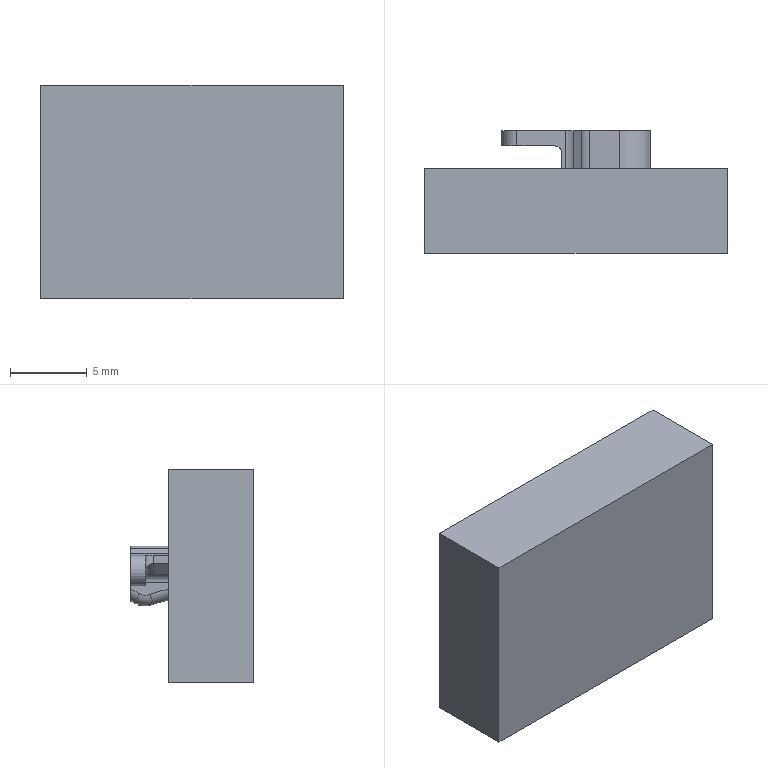NC program | NX | posted with a generic post | part box 19.7 x 8 x 13.91 mm
Lines 9382 to 10432 of 12778:
(ZLEVEL_PROFILE_COPY_1_COPY , TOOL : D1)
N18726 T05 M6
N18728 G54
N18730 G17 G0 G90 X-2.867 Y1.455 B0. C0. S7000 M3
N18732 G43 Z30. H5
N18734 Z-0.02
N18736 G94 G1 X-2.98 Y1.337 F1000.
N18738 X-3.008 Y1.313
N18740 X-3.017 Y1.276
N18742 X-3.004 Y1.24
N18744 G2 X-2.95 Y0.861 R1.381 F850.
N18746 G1 Y0.395
N18748 X-2.095
N18750 X-2.058 Y0.392
N18752 X-2.025 Y0.411
N18754 X-2.009 Y0.445
N18756 X-1.922 Y0.595
N18758 G0 X-2.862 Y1.454 Z-0.04
N18760 G1 X-2.976 Y1.338 F1000.
N18762 X-3.005 Y1.313
N18764 X-3.015 Y1.276
N18766 X-3.001 Y1.241
N18768 G2 X-2.95 Y0.872 R1.386 F850.
N18770 G1 Y0.395
N18772 X-2.095
N18774 X-2.058 Y0.392
N18776 X-2.025 Y0.411
N18778 X-2.009 Y0.445
N18780 X-1.922 Y0.595
N18782 G0 X-2.858 Y1.453 Z-0.06
N18784 G1 X-2.973 Y1.338 F1000.
N18786 X-3.002 Y1.313
N18788 X-3.012 Y1.276
N18790 X-2.999 Y1.241
N18792 G2 X-2.95 Y0.883 R1.392 F850.
N18794 G1 Y0.395
N18796 X-2.095
N18798 X-2.058 Y0.392
N18800 X-2.025 Y0.411
N18802 X-2.009 Y0.445
N18804 X-1.922 Y0.595
N18806 G0 X-2.853 Y1.452 Z-0.08
N18808 G1 X-2.969 Y1.338 F1000.
N18810 X-2.998 Y1.314
N18812 X-3.008 Y1.277
N18814 X-2.995 Y1.241
N18816 G2 X-2.95 Y0.893 R1.365 F850.
N18818 G1 Y0.395
N18820 X-2.095
N18822 X-2.058 Y0.392
N18824 X-2.025 Y0.411
N18826 X-2.009 Y0.445
N18828 X-1.922 Y0.595
N18830 G0 X-2.85 Y1.452 Z-0.1
N18832 G1 X-2.966 Y1.338 F1000.
N18834 X-2.996 Y1.314
N18836 X-3.006 Y1.277
N18838 X-2.993 Y1.241
N18840 G2 X-2.95 Y0.904 R1.396 F850.
N18842 G1 Y0.395
N18844 X-2.095
N18846 X-2.058 Y0.392
N18848 X-2.025 Y0.411
N18850 X-2.009 Y0.445
N18852 X-1.922 Y0.595
N18854 G0 X-2.845 Y1.451 Z-0.12
N18856 G1 X-2.963 Y1.338 F1000.
N18858 X-2.992 Y1.314
N18860 X-3.003 Y1.277
N18862 X-2.991 Y1.242
N18864 G2 X-2.95 Y0.915 R1.401 F850.
N18866 G1 Y0.395
N18868 X-2.095
N18870 X-2.058 Y0.392
N18872 X-2.025 Y0.411
N18874 X-2.009 Y0.445
N18876 X-1.922 Y0.595
N18878 G0 X-2.841 Y1.45 Z-0.14
N18880 G1 X-2.96 Y1.338 F1000.
N18882 X-2.989 Y1.314
N18884 X-3. Y1.278
N18886 X-2.988 Y1.242
N18888 G2 X-2.95 Y0.926 R1.398 F850.
N18890 G1 Y0.395
N18892 X-2.095
N18894 X-2.058 Y0.392
N18896 X-2.025 Y0.411
N18898 X-2.009 Y0.445
N18900 X-1.922 Y0.595
N18902 G0 X-2.837 Y1.449 Z-0.16
N18904 G1 X-2.956 Y1.338 F1000.
N18906 X-2.986 Y1.315
N18908 X-2.997 Y1.278
N18910 X-2.985 Y1.242
N18912 G2 X-2.95 Y0.937 R1.395 F850.
N18914 G1 Y0.395
N18916 X-2.095
N18918 X-2.058 Y0.392
N18920 X-2.025 Y0.411
N18922 X-2.009 Y0.445
N18924 X-1.922 Y0.595
N18926 G0 X-2.833 Y1.448 Z-0.18
N18928 G1 X-2.953 Y1.338 F1000.
N18930 X-2.983 Y1.315
N18932 X-2.994 Y1.278
N18934 X-2.983 Y1.242
N18936 G2 X-2.95 Y0.948 R1.391 F850.
N18938 G1 Y0.395
N18940 X-2.095
N18942 X-2.058 Y0.392
N18944 X-2.025 Y0.411
N18946 X-2.009 Y0.445
N18948 X-1.922 Y0.595
N18950 G0 X-2.828 Y1.447 Z-0.2
N18952 G1 X-2.949 Y1.338 F1000.
N18954 X-2.979 Y1.315
N18956 X-2.991 Y1.279
N18958 X-2.98 Y1.243
N18960 G2 X-2.95 Y0.959 R1.369 F850.
N18962 G1 Y0.395
N18964 X-2.095
N18966 X-2.058 Y0.392
N18968 X-2.025 Y0.411
N18970 X-2.009 Y0.445
N18972 X-1.922 Y0.595
N18974 G0 X-2.824 Y1.445 Z-0.22
N18976 G1 X-2.946 Y1.338 F1000.
N18978 X-2.977 Y1.315
N18980 X-2.989 Y1.279
N18982 X-2.978 Y1.243
N18984 G2 X-2.95 Y0.97 R1.379 F850.
N18986 G1 Y0.395
N18988 X-2.095
N18990 X-2.058 Y0.392
N18992 X-2.025 Y0.411
N18994 X-2.009 Y0.445
N18996 X-1.922 Y0.595
N18998 G0 X-2.82 Y1.444 Z-0.24
N19000 G1 X-2.943 Y1.337 F1000.
N19002 X-2.974 Y1.315
N19004 X-2.986 Y1.279
N19006 X-2.976 Y1.243
N19008 G2 X-2.95 Y0.981 R1.376 F850.
N19010 G1 Y0.395
N19012 X-2.095
N19014 X-2.058 Y0.392
N19016 X-2.025 Y0.411
N19018 X-2.009 Y0.445
N19020 X-1.922 Y0.595
N19022 G0 X-2.817 Y1.443 Z-0.26
N19024 G1 X-2.94 Y1.337 F1000.
N19026 X-2.971 Y1.315
N19028 X-2.984 Y1.279
N19030 X-2.973 Y1.243
N19032 G2 X-2.95 Y0.992 R1.374 F850.
N19034 G1 Y0.395
N19036 X-2.095
N19038 X-2.058 Y0.392
N19040 X-2.025 Y0.411
N19042 X-2.009 Y0.445
N19044 X-1.922 Y0.595
N19046 G0 X-2.813 Y1.442 Z-0.28
N19048 G1 X-2.938 Y1.337 F1000.
N19050 X-2.969 Y1.315
N19052 X-2.981 Y1.279
N19054 X-2.972 Y1.243
N19056 G2 X-2.95 Y1.003 R1.375 F850.
N19058 G1 Y0.395
N19060 X-2.095
N19062 X-2.058 Y0.392
N19064 X-2.025 Y0.411
N19066 X-2.009 Y0.445
N19068 X-1.922 Y0.595
N19070 G0 X-2.808 Y1.44 Z-0.3
N19072 G1 X-2.933 Y1.337 F1000.
N19074 X-2.965 Y1.315
N19076 X-2.978 Y1.28
N19078 X-2.968 Y1.243
N19080 G2 X-2.95 Y1.014 R1.335 F850.
N19082 G1 Y0.395
N19084 X-2.095
N19086 X-2.058 Y0.392
N19088 X-2.025 Y0.411
N19090 X-2.009 Y0.445
N19092 X-1.922 Y0.595
N19094 G0 X-2.805 Y1.439 Z-0.32
N19096 G1 X-2.931 Y1.337 F1000.
N19098 X-2.962 Y1.316
N19100 X-2.976 Y1.28
N19102 X-2.967 Y1.243
N19104 G2 X-2.95 Y1.025 R1.337 F850.
N19106 G1 Y0.395
N19108 X-2.095
N19110 X-2.058 Y0.392
N19112 X-2.025 Y0.411
N19114 X-2.009 Y0.445
N19116 X-1.922 Y0.595
N19118 G0 X-2.804 Y1.439 Z-0.34
N19120 G1 X-2.93 Y1.337 F1000.
N19122 X-2.962 Y1.316
N19124 X-2.976 Y1.28
N19126 X-2.967 Y1.243
N19128 G2 X-2.95 Y1.036 R1.382 F850.
N19130 G1 Y0.395
N19132 X-2.095
N19134 X-2.058 Y0.392
N19136 X-2.025 Y0.411
N19138 X-2.009 Y0.445
N19140 X-1.922 Y0.595
N19142 G0 X-2.801 Y1.438 Z-0.36
N19144 G1 X-2.928 Y1.336 F1000.
N19146 X-2.96 Y1.316
N19148 X-2.974 Y1.28
N19150 X-2.965 Y1.243
N19152 X-2.944 Y1.146 F850.
N19154 X-2.95 Y1.047
N19156 Y0.395
N19158 X-2.095
N19160 X-2.058 Y0.392
N19162 X-2.025 Y0.411
N19164 X-2.009 Y0.445
N19166 X-1.922 Y0.595
N19168 G0 X-2.797 Y1.436 Z-0.38
N19170 G1 X-2.926 Y1.336 F1000.
N19172 X-2.957 Y1.316
N19174 X-2.972 Y1.28
N19176 X-2.963 Y1.243
N19178 X-2.944 Y1.151 F850.
N19180 X-2.95 Y1.058
N19182 Y0.395
N19184 X-2.095
N19186 X-2.058 Y0.392
N19188 X-2.025 Y0.411
N19190 X-2.009 Y0.445
N19192 X-1.922 Y0.595
N19194 G0 X-2.794 Y1.435 Z-0.4
N19196 G1 X-2.923 Y1.336 F1000.
N19198 X-2.955 Y1.316
N19200 X-2.97 Y1.28
N19202 X-2.961 Y1.243
N19204 X-2.943 Y1.157 F850.
N19206 X-2.95 Y1.069
N19208 Y0.395
N19210 X-2.095
N19212 X-2.058 Y0.392
N19214 X-2.025 Y0.411
N19216 X-2.009 Y0.445
N19218 X-1.922 Y0.595
N19220 G0 X-2.79 Y1.433 Z-0.42
N19222 G1 X-2.92 Y1.335 F1000.
N19224 X-2.952 Y1.316
N19226 X-2.967 Y1.28
N19228 X-2.959 Y1.244
N19230 X-2.942 Y1.162 F850.
N19232 X-2.95 Y1.079
N19234 Y0.395
N19236 X-2.095
N19238 X-2.058 Y0.392
N19240 X-2.025 Y0.411
N19242 X-2.009 Y0.445
N19244 X-1.922 Y0.595
N19246 G0 X-2.788 Y1.432 Z-0.44
N19248 G1 X-2.919 Y1.335 F1000.
N19250 X-2.951 Y1.316
N19252 X-2.966 Y1.281
N19254 X-2.958 Y1.244
N19256 X-2.95 Y1.09 F850.
N19258 Y0.395
N19260 X-2.095
N19262 X-2.058 Y0.392
N19264 X-2.025 Y0.411
N19266 X-2.009 Y0.445
N19268 X-1.922 Y0.595
N19270 G0 X-2.785 Y1.431 Z-0.46
N19272 G1 X-2.917 Y1.335 F1000.
N19274 X-2.949 Y1.316
N19276 X-2.965 Y1.281
N19278 X-2.957 Y1.244
N19280 X-2.95 Y1.101 F850.
N19282 Y0.395
N19284 X-2.095
N19286 X-2.058 Y0.392
N19288 X-2.025 Y0.411
N19290 X-2.009 Y0.445
N19292 X-1.922 Y0.595
N19294 G0 X-2.783 Y1.429 Z-0.48
N19296 G1 X-2.915 Y1.335 F1000.
N19298 X-2.948 Y1.316
N19300 X-2.963 Y1.281
N19302 X-2.956 Y1.244
N19304 X-2.95 Y1.112 F850.
N19306 Y0.395
N19308 X-2.095
N19310 X-2.058 Y0.392
N19312 X-2.025 Y0.411
N19314 X-2.009 Y0.445
N19316 X-1.922 Y0.595
N19318 G0 X-2.781 Y1.428 Z-0.5
N19320 G1 X-2.914 Y1.334 F1000.
N19322 X-2.946 Y1.315
N19324 X-2.962 Y1.281
N19326 X-2.956 Y1.244
N19328 X-2.95 Y1.123 F850.
N19330 Y0.395
N19332 X-2.095
N19334 X-2.058 Y0.392
N19336 X-2.025 Y0.411
N19338 X-2.009 Y0.445
N19340 X-1.922 Y0.595
N19342 G0 X-2.778 Y1.426 Z-0.52
N19344 G1 X-2.912 Y1.334 F1000.
N19346 X-2.944 Y1.315
N19348 X-2.961 Y1.281
N19350 X-2.954 Y1.244
N19352 X-2.95 Y1.134 F850.
N19354 Y0.395
N19356 X-2.095
N19358 X-2.058 Y0.392
N19360 X-2.025 Y0.411
N19362 X-2.009 Y0.445
N19364 X-1.922 Y0.595
N19366 G0 X-2.776 Y1.425 Z-0.54
N19368 G1 X-2.91 Y1.334 F1000.
N19370 X-2.943 Y1.315
N19372 X-2.96 Y1.281
N19374 X-2.954 Y1.244
N19376 X-2.95 Y1.145 F850.
N19378 Y0.395
N19380 X-2.095
N19382 X-2.058 Y0.392
N19384 X-2.025 Y0.411
N19386 X-2.009 Y0.445
N19388 X-1.922 Y0.595
N19390 G0 X-2.775 Y1.425 Z-0.56
N19392 G1 X-2.91 Y1.334 F1000.
N19394 X-2.943 Y1.315
N19396 X-2.959 Y1.281
N19398 X-2.953 Y1.244
N19400 X-2.95 Y1.156 F850.
N19402 Y0.395
N19404 X-2.095
N19406 X-2.058 Y0.392
N19408 X-2.025 Y0.411
N19410 X-2.009 Y0.445
N19412 X-1.922 Y0.595
N19414 G0 X-2.774 Y1.424 Z-0.58
N19416 G1 X-2.909 Y1.334 F1000.
N19418 X-2.942 Y1.315
N19420 X-2.959 Y1.281
N19422 X-2.953 Y1.244
N19424 X-2.95 Y1.166 F850.
N19426 Y0.395
N19428 X-2.095
N19430 X-2.058 Y0.392
N19432 X-2.025 Y0.411
N19434 X-2.009 Y0.445
N19436 X-1.922 Y0.595
N19438 G0 X-2.772 Y1.429 Z-0.6
N19440 G1 X-2.912 Y1.334 F1000.
N19442 X-2.945 Y1.315
N19444 X-2.961 Y1.281
N19446 X-2.955 Y1.244
N19448 X-2.95 Y1.176 F850.
N19450 Y0.395
N19452 X-2.095
N19454 X-2.058 Y0.392
N19456 X-2.025 Y0.411
N19458 X-2.009 Y0.445
N19460 X-1.922 Y0.595
N19462 G0 X-2.774 Y1.432 Z-0.62
N19464 G1 X-2.913 Y1.334 F1000.
N19466 X-2.946 Y1.316
N19468 X-2.962 Y1.281
N19470 X-2.955 Y1.244
N19472 X-2.95 Y1.186 F850.
N19474 Y0.395
N19476 X-2.095
N19478 X-2.058 Y0.392
N19480 X-2.025 Y0.411
N19482 X-2.009 Y0.445
N19484 X-1.922 Y0.595
N19486 G0 X-2.767 Y1.409 Z-0.64
N19488 G1 X-2.903 Y1.33 F1000.
N19490 X-2.938 Y1.315
N19492 X-2.957 Y1.281
N19494 X-2.953 Y1.244
N19496 Y1.222 F850.
N19498 X-2.95 Y1.195
N19500 Y0.395
N19502 X-2.095
N19504 X-2.058 Y0.392
N19506 X-2.025 Y0.411
N19508 X-2.009 Y0.445
N19510 X-1.922 Y0.595
N19512 G0 X-2.766 Y1.41 Z-0.66
N19514 G1 X-2.903 Y1.33 F1000.
N19516 X-2.938 Y1.315
N19518 X-2.957 Y1.281
N19520 X-2.953 Y1.244
N19522 Y1.222 F850.
N19524 X-2.95 Y1.203
N19526 Y0.395
N19528 X-2.095
N19530 X-2.058 Y0.392
N19532 X-2.025 Y0.411
N19534 X-2.009 Y0.445
N19536 X-1.922 Y0.595
N19538 G0 X-2.765 Y1.416 Z-0.68
N19540 G1 X-2.903 Y1.332 F1000.
N19542 X-2.937 Y1.315
N19544 X-2.955 Y1.281
N19546 X-2.95 Y1.244
N19548 Y1.211 F850.
N19550 Y0.395
N19552 X-2.095
N19554 X-2.058 Y0.392
N19556 X-2.025 Y0.411
N19558 X-2.009 Y0.445
N19560 X-1.922 Y0.595
N19562 G0 X-2.764 Y1.416 Z-0.7
N19564 G1 X-2.902 Y1.332 F1000.
N19566 X-2.936 Y1.315
N19568 X-2.955 Y1.281
N19570 X-2.95 Y1.244
N19572 Y1.218 F850.
N19574 Y0.395
N19576 X-2.095
N19578 X-2.058 Y0.392
N19580 X-2.025 Y0.411
N19582 X-2.009 Y0.445
N19584 X-1.922 Y0.595
N19586 G0 X-2.767 Y1.432 Z-0.72
N19588 G1 X-2.909 Y1.334 F1000.
N19590 X-2.942 Y1.316
N19592 X-2.958 Y1.281
N19594 X-2.952 Y1.244
N19596 X-2.95 Y1.225 F850.
N19598 Y0.395
N19600 X-2.095
N19602 X-2.058 Y0.392
N19604 X-2.025 Y0.411
N19606 X-2.009 Y0.445
N19608 X-1.922 Y0.595
N19610 G0 X-2.77 Y1.461 Z-0.74
N19612 G1 X-2.918 Y1.338 F1000.
N19614 X-2.949 Y1.316
N19616 X-2.962 Y1.28
N19618 X-2.952 Y1.244
N19620 X-2.95 Y1.231 F850.
N19622 Y0.395
N19624 X-2.095
N19626 X-2.058 Y0.392
N19628 X-2.025 Y0.411
N19630 X-2.009 Y0.445
N19632 X-1.922 Y0.595
N19634 G0 X-2.761 Y1.413 Z-0.76
N19636 G1 X-2.901 Y1.331 F1000.
N19638 X-2.935 Y1.315
N19640 X-2.954 Y1.282
N19642 X-2.95 Y1.244
N19644 Y0.395 F850.
N19646 X-2.095
N19648 X-2.058 Y0.392
N19650 X-2.025 Y0.411
N19652 X-2.009 Y0.445
N19654 X-1.922 Y0.595
N19656 G0 X-2.761 Y1.412 Z-0.78
N19658 G1 X-2.9 Y1.331 F1000.
N19660 X-2.935 Y1.315
N19662 X-2.954 Y1.282
N19664 X-2.95 Y1.244
N19666 Y0.395 F850.
N19668 X-2.095
N19670 X-2.058 Y0.392
N19672 X-2.025 Y0.411
N19674 X-2.009 Y0.445
N19676 X-1.922 Y0.595
N19678 G0 X-2.76 Y1.411 Z-0.8
N19680 G1 X-2.9 Y1.331 F1000.
N19682 X-2.934 Y1.315
N19684 X-2.953 Y1.282
N19686 X-2.95 Y1.244
N19688 Y0.395 F850.
N19690 X-2.095
N19692 X-2.058 Y0.392
N19694 X-2.025 Y0.411
N19696 X-2.009 Y0.445
N19698 X-1.922 Y0.595
N19700 G0 X-2.76 Y1.411 Z-0.82
N19702 G1 X-2.9 Y1.331 F1000.
N19704 X-2.934 Y1.315
N19706 X-2.953 Y1.282
N19708 X-2.95 Y1.244
N19710 Y0.395 F850.
N19712 X-2.095
N19714 X-2.058 Y0.392
N19716 X-2.025 Y0.411
N19718 X-2.009 Y0.445
N19720 X-1.922 Y0.595
N19722 G0 X-2.76 Y1.412 Z-0.84
N19724 G1 X-2.9 Y1.331 F1000.
N19726 X-2.934 Y1.315
N19728 X-2.953 Y1.282
N19730 X-2.95 Y1.244
N19732 Y0.395 F850.
N19734 X-2.095
N19736 X-2.058 Y0.392
N19738 X-2.025 Y0.411
N19740 X-2.009 Y0.445
N19742 X-1.922 Y0.595
N19744 G0 X-2.76 Y1.412 Z-0.86
N19746 G1 X-2.9 Y1.331 F1000.
N19748 X-2.934 Y1.315
N19750 X-2.953 Y1.282
N19752 X-2.95 Y1.244
N19754 Y0.395 F850.
N19756 X-2.095
N19758 X-2.058 Y0.392
N19760 X-2.025 Y0.411
N19762 X-2.009 Y0.445
N19764 X-1.922 Y0.595
N19766 G0 X-2.76 Y1.412 Z-0.88
N19768 G1 X-2.9 Y1.331 F1000.
N19770 X-2.934 Y1.315
N19772 X-2.953 Y1.282
N19774 X-2.95 Y1.244
N19776 Y0.395 F850.
N19778 X-2.095
N19780 X-2.058 Y0.392
N19782 X-2.025 Y0.411
N19784 X-2.009 Y0.445
N19786 X-1.922 Y0.595
N19788 G0 X-2.76 Y1.412 Z-0.9
N19790 G1 X-2.9 Y1.331 F1000.
N19792 X-2.934 Y1.315
N19794 X-2.953 Y1.282
N19796 X-2.95 Y1.244
N19798 Y0.395 F850.
N19800 X-2.095
N19802 X-2.058 Y0.392
N19804 X-2.024 Y0.411
N19806 X-2.009 Y0.445
N19808 X-1.922 Y0.595
N19810 G0 X-2.76 Y1.412 Z-0.92
N19812 G1 X-2.9 Y1.331 F1000.
N19814 X-2.934 Y1.315
N19816 X-2.953 Y1.282
N19818 X-2.95 Y1.244
N19820 Y0.395 F850.
N19822 X-2.095
N19824 X-2.058 Y0.392
N19826 X-2.024 Y0.411
N19828 X-2.009 Y0.445
N19830 X-1.922 Y0.595
N19832 G0 X-2.76 Y1.412 Z-0.94
N19834 G1 X-2.9 Y1.331 F1000.
N19836 X-2.934 Y1.315
N19838 X-2.953 Y1.282
N19840 X-2.95 Y1.244
N19842 Y0.395 F850.
N19844 X-2.095
N19846 X-2.058 Y0.392
N19848 X-2.024 Y0.411
N19850 X-2.009 Y0.445
N19852 X-1.922 Y0.595
N19854 G0 X-2.76 Y1.412 Z-0.96
N19856 G1 X-2.9 Y1.331 F1000.
N19858 X-2.934 Y1.315
N19860 X-2.953 Y1.282
N19862 X-2.95 Y1.244
N19864 Y0.395 F850.
N19866 X-2.095
N19868 X-2.058 Y0.392
N19870 X-2.024 Y0.411
N19872 X-2.009 Y0.445
N19874 X-1.922 Y0.595
N19876 G0 X-2.76 Y1.412 Z-0.98
N19878 G1 X-2.9 Y1.331 F1000.
N19880 X-2.934 Y1.315
N19882 X-2.953 Y1.282
N19884 X-2.95 Y1.244
N19886 Y0.395 F850.
N19888 X-2.095
N19890 X-2.058 Y0.392
N19892 X-2.024 Y0.411
N19894 X-2.009 Y0.445
N19896 X-1.922 Y0.595
N19898 G0 X-2.76 Y1.412 Z-1.
N19900 G1 X-2.9 Y1.331 F1000.
N19902 X-2.934 Y1.315
N19904 X-2.953 Y1.282
N19906 X-2.95 Y1.244
N19908 Y0.395 F850.
N19910 X-2.095
N19912 X-2.058 Y0.392
N19914 X-2.024 Y0.411
N19916 X-2.009 Y0.445
N19918 X-1.922 Y0.595
N19920 G0 X-2.76 Y1.412 Z-1.02
N19922 G1 X-2.9 Y1.331 F1000.
N19924 X-2.934 Y1.315
N19926 X-2.953 Y1.282
N19928 X-2.95 Y1.244
N19930 Y0.395 F850.
N19932 X-2.095
N19934 X-2.058 Y0.392
N19936 X-2.024 Y0.411
N19938 X-2.009 Y0.445
N19940 X-1.922 Y0.595
N19942 G0 X-2.76 Y1.412 Z-1.04
N19944 G1 X-2.9 Y1.331 F1000.
N19946 X-2.934 Y1.315
N19948 X-2.953 Y1.282
N19950 X-2.95 Y1.244
N19952 Y0.395 F850.
N19954 X-2.095
N19956 X-2.058 Y0.392
N19958 X-2.024 Y0.411
N19960 X-2.009 Y0.445
N19962 X-1.922 Y0.595
N19964 G0 X-2.76 Y1.412 Z-1.06
N19966 G1 X-2.9 Y1.331 F1000.
N19968 X-2.934 Y1.315
N19970 X-2.953 Y1.282
N19972 X-2.95 Y1.244
N19974 Y0.395 F850.
N19976 X-2.095
N19978 X-2.058 Y0.392
N19980 X-2.024 Y0.411
N19982 X-2.009 Y0.445
N19984 X-1.922 Y0.595
N19986 G0 X-2.76 Y1.412 Z-1.08
N19988 G1 X-2.9 Y1.331 F1000.
N19990 X-2.934 Y1.315
N19992 X-2.953 Y1.282
N19994 X-2.95 Y1.244
N19996 Y0.395 F850.
N19998 X-2.095
N20000 X-2.058 Y0.392
N20002 X-2.024 Y0.411
N20004 X-2.009 Y0.445
N20006 X-1.922 Y0.595
N20008 G0 X-2.76 Y1.411 Z-1.1
N20010 G1 X-2.9 Y1.331 F1000.
N20012 X-2.934 Y1.315
N20014 X-2.953 Y1.282
N20016 X-2.95 Y1.244
N20018 Y0.395 F850.
N20020 X-2.095
N20022 X-2.058 Y0.392
N20024 X-2.024 Y0.411
N20026 X-2.009 Y0.445
N20028 X-1.922 Y0.595
N20030 G0 X-2.76 Y1.411 Z-1.12
N20032 G1 X-2.9 Y1.331 F1000.
N20034 X-2.934 Y1.315
N20036 X-2.953 Y1.282
N20038 X-2.95 Y1.244
N20040 Y0.395 F850.
N20042 X-2.095
N20044 X-2.058 Y0.392
N20046 X-2.024 Y0.411
N20048 X-2.009 Y0.445
N20050 X-1.922 Y0.595
N20052 G0 X-2.76 Y1.411 Z-1.14
N20054 G1 X-2.9 Y1.331 F1000.
N20056 X-2.934 Y1.315
N20058 X-2.953 Y1.282
N20060 X-2.95 Y1.244
N20062 Y0.395 F850.
N20064 X-2.095
N20066 X-2.058 Y0.392
N20068 X-2.024 Y0.411
N20070 X-2.009 Y0.445
N20072 X-1.922 Y0.595
N20074 G0 X-2.76 Y1.411 Z-1.16
N20076 G1 X-2.9 Y1.331 F1000.
N20078 X-2.934 Y1.315
N20080 X-2.953 Y1.282
N20082 X-2.95 Y1.244
N20084 Y0.395 F850.
N20086 X-2.095
N20088 X-2.058 Y0.392
N20090 X-2.024 Y0.411
N20092 X-2.009 Y0.445
N20094 X-1.922 Y0.595
N20096 G0 X-2.76 Y1.411 Z-1.18
N20098 G1 X-2.9 Y1.331 F1000.
N20100 X-2.934 Y1.315
N20102 X-2.953 Y1.282
N20104 X-2.95 Y1.244
N20106 Y0.395 F850.
N20108 X-2.095
N20110 X-2.058 Y0.392
N20112 X-2.024 Y0.411
N20114 X-2.009 Y0.445
N20116 X-1.922 Y0.595
N20118 G0 X-2.76 Y1.411 Z-1.2
N20120 G1 X-2.9 Y1.331 F1000.
N20122 X-2.934 Y1.315
N20124 X-2.953 Y1.282
N20126 X-2.95 Y1.244
N20128 Y0.395 F850.
N20130 X-2.095
N20132 X-2.058 Y0.392
N20134 X-2.024 Y0.411
N20136 X-2.009 Y0.445
N20138 X-1.922 Y0.595
N20140 G0 X-2.76 Y1.411 Z-1.22
N20142 G1 X-2.9 Y1.331 F1000.
N20144 X-2.934 Y1.315
N20146 X-2.953 Y1.282
N20148 X-2.95 Y1.244
N20150 Y0.395 F850.
N20152 X-2.095
N20154 X-2.057 Y0.392
N20156 X-2.024 Y0.411
N20158 X-2.009 Y0.445
N20160 X-1.922 Y0.595
N20162 G0 X-2.76 Y1.411 Z-1.24
N20164 G1 X-2.9 Y1.331 F1000.
N20166 X-2.934 Y1.315
N20168 X-2.953 Y1.282
N20170 X-2.95 Y1.244
N20172 Y0.395 F850.
N20174 X-2.095
N20176 X-2.057 Y0.392
N20178 X-2.024 Y0.411
N20180 X-2.009 Y0.445
N20182 X-1.922 Y0.595
N20184 G0 X-2.76 Y1.411 Z-1.26
N20186 G1 X-2.9 Y1.331 F1000.
N20188 X-2.934 Y1.315
N20190 X-2.953 Y1.282
N20192 X-2.95 Y1.244
N20194 Y0.395 F850.
N20196 X-2.095
N20198 X-2.057 Y0.392
N20200 X-2.024 Y0.411
N20202 X-2.009 Y0.445
N20204 X-1.922 Y0.595
N20206 G0 X-2.76 Y1.411 Z-1.28
N20208 G1 X-2.9 Y1.331 F1000.
N20210 X-2.934 Y1.315
N20212 X-2.953 Y1.282
N20214 X-2.95 Y1.244
N20216 Y0.395 F850.
N20218 X-2.095
N20220 X-2.057 Y0.392
N20222 X-2.024 Y0.411
N20224 X-2.008 Y0.445
N20226 X-1.922 Y0.595
N20228 G0 X-2.76 Y1.411 Z-1.3
N20230 G1 X-2.9 Y1.331 F1000.
N20232 X-2.934 Y1.315
N20234 X-2.953 Y1.282
N20236 X-2.95 Y1.244
N20238 Y0.395 F850.
N20240 X-2.095
N20242 X-2.057 Y0.392
N20244 X-2.024 Y0.411
N20246 X-2.008 Y0.445
N20248 X-1.922 Y0.595
N20250 G0 X-2.76 Y1.411 Z-1.32
N20252 G1 X-2.9 Y1.331 F1000.
N20254 X-2.934 Y1.315
N20256 X-2.953 Y1.282
N20258 X-2.95 Y1.244
N20260 Y0.395 F850.
N20262 X-2.095
N20264 X-2.057 Y0.392
N20266 X-2.024 Y0.411
N20268 X-2.008 Y0.445
N20270 X-1.922 Y0.595
N20272 G0 X-2.76 Y1.411 Z-1.34
N20274 G1 X-2.9 Y1.331 F1000.
N20276 X-2.934 Y1.315
N20278 X-2.953 Y1.282
N20280 X-2.95 Y1.244
N20282 Y0.395 F850.
N20284 X-2.095
N20286 X-2.057 Y0.392
N20288 X-2.024 Y0.411
N20290 X-2.008 Y0.445
N20292 X-1.922 Y0.595
N20294 G0 X-2.76 Y1.411 Z-1.36
N20296 G1 X-2.9 Y1.331 F1000.
N20298 X-2.934 Y1.315
N20300 X-2.953 Y1.282
N20302 X-2.95 Y1.244
N20304 Y0.395 F850.
N20306 X-2.095
N20308 X-2.057 Y0.392
N20310 X-2.024 Y0.411
N20312 X-2.008 Y0.445
N20314 X-1.922 Y0.595
N20316 G0 X-2.76 Y1.411 Z-1.38
N20318 G1 X-2.9 Y1.331 F1000.
N20320 X-2.934 Y1.315
N20322 X-2.953 Y1.282
N20324 X-2.95 Y1.244
N20326 Y0.395 F850.
N20328 X-2.095
N20330 X-2.057 Y0.392
N20332 X-2.024 Y0.411
N20334 X-2.008 Y0.445
N20336 X-1.922 Y0.595
N20338 G0 X-2.76 Y1.411 Z-1.4
N20340 G1 X-2.9 Y1.331 F1000.
N20342 X-2.934 Y1.315
N20344 X-2.953 Y1.282
N20346 X-2.95 Y1.244
N20348 Y0.395 F850.
N20350 X-2.095
N20352 X-2.057 Y0.392
N20354 X-2.024 Y0.411
N20356 X-2.008 Y0.445
N20358 X-1.922 Y0.595
N20360 G0 X-2.76 Y1.411 Z-1.42
N20362 G1 X-2.9 Y1.331 F1000.
N20364 X-2.934 Y1.315
N20366 X-2.953 Y1.282
N20368 X-2.95 Y1.244
N20370 Y0.395 F850.
N20372 X-2.095
N20374 X-2.057 Y0.392
N20376 X-2.024 Y0.411
N20378 X-2.008 Y0.445
N20380 X-1.922 Y0.595
N20382 G0 X-2.76 Y1.412 Z-1.44
N20384 G1 X-2.9 Y1.331 F1000.
N20386 X-2.934 Y1.315
N20388 X-2.953 Y1.282
N20390 X-2.95 Y1.245
N20392 Y0.395 F850.
N20394 X-2.095
N20396 X-2.057 Y0.392
N20398 X-2.024 Y0.411
N20400 X-2.008 Y0.445
N20402 X-1.922 Y0.595
N20404 G0 X-2.76 Y1.412 Z-1.46
N20406 G1 X-2.9 Y1.331 F1000.
N20408 X-2.934 Y1.315
N20410 X-2.953 Y1.282
N20412 X-2.95 Y1.245
N20414 Y0.395 F850.
N20416 X-2.095
N20418 X-2.057 Y0.392
N20420 X-2.024 Y0.411
N20422 X-2.008 Y0.445
N20424 X-1.922 Y0.595
N20426 G0 X-2.76 Y1.412 Z-1.48
N20428 G1 X-2.9 Y1.331 F1000.
N20430 X-2.934 Y1.315
N20432 X-2.953 Y1.282
N20434 X-2.95 Y1.245
N20436 Y0.395 F850.
N20438 X-2.095
N20440 X-2.057 Y0.392
N20442 X-2.024 Y0.411
N20444 X-2.008 Y0.445
N20446 X-1.922 Y0.595
N20448 G0 X-2.76 Y1.412 Z-1.5
N20450 G1 X-2.9 Y1.331 F1000.
N20452 X-2.934 Y1.315
N20454 X-2.953 Y1.282
N20456 X-2.95 Y1.245
N20458 Y0.395 F850.
N20460 X-2.095
N20462 X-2.057 Y0.392
N20464 X-2.024 Y0.411
N20466 X-2.008 Y0.445
N20468 X-1.922 Y0.595
N20470 G0 X-2.76 Y1.412 Z-1.52
N20472 G1 X-2.9 Y1.331 F1000.
N20474 X-2.934 Y1.315
N20476 X-2.953 Y1.282
N20478 X-2.95 Y1.245
N20480 Y0.395 F850.
N20482 X-2.095
N20484 X-2.057 Y0.392
N20486 X-2.024 Y0.411
N20488 X-2.008 Y0.445
N20490 X-1.922 Y0.595
N20492 G0 X-2.76 Y1.412 Z-1.54
N20494 G1 X-2.9 Y1.331 F1000.
N20496 X-2.934 Y1.315
N20498 X-2.953 Y1.282
N20500 X-2.95 Y1.245
N20502 Y0.395 F850.
N20504 X-2.095
N20506 X-2.057 Y0.392
N20508 X-2.024 Y0.411
N20510 X-2.008 Y0.445
N20512 X-1.922 Y0.595
N20514 G0 X-2.76 Y1.412 Z-1.56
N20516 G1 X-2.9 Y1.331 F1000.
N20518 X-2.934 Y1.315
N20520 X-2.953 Y1.282
N20522 X-2.95 Y1.245
N20524 Y0.395 F850.
N20526 X-2.095
N20528 X-2.057 Y0.392
N20530 X-2.024 Y0.411
N20532 X-2.008 Y0.445
N20534 X-1.922 Y0.595
N20536 G0 X-2.76 Y1.412 Z-1.58
N20538 G1 X-2.9 Y1.331 F1000.
N20540 X-2.934 Y1.315
N20542 X-2.953 Y1.282
N20544 X-2.95 Y1.245
N20546 Y0.395 F850.
N20548 X-2.095
N20550 X-2.057 Y0.392
N20552 X-2.024 Y0.411
N20554 X-2.008 Y0.445
N20556 X-1.922 Y0.595
N20558 G0 X-2.76 Y1.412 Z-1.6
N20560 G1 X-2.9 Y1.331 F1000.
N20562 X-2.934 Y1.315
N20564 X-2.953 Y1.282
N20566 X-2.95 Y1.245
N20568 Y0.395 F850.
N20570 X-2.095
N20572 X-2.057 Y0.392
N20574 X-2.024 Y0.411
N20576 X-2.008 Y0.445
N20578 X-1.922 Y0.595
N20580 G0 X-2.76 Y1.412 Z-1.62
N20582 G1 X-2.9 Y1.331 F1000.
N20584 X-2.934 Y1.315
N20586 X-2.953 Y1.282
N20588 X-2.95 Y1.245
N20590 Y0.395 F850.
N20592 X-2.095
N20594 X-2.057 Y0.392
N20596 X-2.024 Y0.411
N20598 X-2.008 Y0.445
N20600 X-1.922 Y0.595
N20602 G0 X-2.76 Y1.412 Z-1.64
N20604 G1 X-2.9 Y1.331 F1000.
N20606 X-2.934 Y1.315
N20608 X-2.953 Y1.282
N20610 X-2.95 Y1.245
N20612 Y0.395 F850.
N20614 X-2.095
N20616 X-2.057 Y0.392
N20618 X-2.024 Y0.411
N20620 X-2.008 Y0.445
N20622 X-1.922 Y0.595
N20624 G0 X-2.76 Y1.412 Z-1.66
N20626 G1 X-2.9 Y1.331 F1000.
N20628 X-2.934 Y1.315
N20630 X-2.953 Y1.282
N20632 X-2.95 Y1.245
N20634 Y0.395 F850.
N20636 X-2.095
N20638 X-2.057 Y0.392
N20640 X-2.024 Y0.411
N20642 X-2.008 Y0.445
N20644 X-1.922 Y0.595
N20646 G0 X-2.76 Y1.412 Z-1.68
N20648 G1 X-2.9 Y1.331 F1000.
N20650 X-2.934 Y1.315
N20652 X-2.953 Y1.282
N20654 X-2.95 Y1.245
N20656 Y0.395 F850.
N20658 X-2.095
N20660 X-2.057 Y0.392
N20662 X-2.024 Y0.411
N20664 X-2.008 Y0.445
N20666 X-1.922 Y0.595
N20668 G0 X-2.76 Y1.412 Z-1.7
N20670 G1 X-2.9 Y1.331 F1000.
N20672 X-2.934 Y1.315
N20674 X-2.953 Y1.282
N20676 X-2.95 Y1.245
N20678 Y0.395 F850.
N20680 X-2.095
N20682 X-2.057 Y0.392
N20684 X-2.024 Y0.411
N20686 X-2.008 Y0.445
N20688 X-1.922 Y0.595
N20690 G0 X-2.76 Y1.412 Z-1.72
N20692 G1 X-2.9 Y1.331 F1000.
N20694 X-2.934 Y1.315
N20696 X-2.953 Y1.282
N20698 X-2.95 Y1.245
N20700 Y0.395 F850.
N20702 X-2.095
N20704 X-2.057 Y0.392
N20706 X-2.024 Y0.411
N20708 X-2.008 Y0.445
N20710 X-1.922 Y0.595
N20712 G0 X-2.76 Y1.412 Z-1.74
N20714 G1 X-2.9 Y1.331 F1000.
N20716 X-2.934 Y1.315
N20718 X-2.953 Y1.282
N20720 X-2.95 Y1.245
N20722 Y0.395 F850.
N20724 X-2.095
N20726 X-2.057 Y0.392
N20728 X-2.024 Y0.411
N20730 X-2.008 Y0.445
N20732 X-1.922 Y0.595
N20734 G0 X-2.76 Y1.412 Z-1.76
N20736 G1 X-2.9 Y1.331 F1000.
N20738 X-2.934 Y1.315
N20740 X-2.953 Y1.282
N20742 X-2.95 Y1.245
N20744 Y0.395 F850.
N20746 X-2.095
N20748 X-2.057 Y0.392
N20750 X-2.024 Y0.411
N20752 X-2.008 Y0.445
N20754 X-1.922 Y0.595
N20756 G0 X-2.76 Y1.412 Z-1.78
N20758 G1 X-2.9 Y1.331 F1000.
N20760 X-2.934 Y1.315
N20762 X-2.953 Y1.282
N20764 X-2.95 Y1.245
N20766 Y0.395 F850.
N20768 X-2.095
N20770 X-2.057 Y0.392
N20772 X-2.024 Y0.411
N20774 X-2.008 Y0.445
N20776 X-1.922 Y0.595
N20778 G0 X-2.76 Y1.412 Z-1.8
N20780 G1 X-2.9 Y1.331 F1000.
N20782 X-2.934 Y1.315
N20784 X-2.953 Y1.282
N20786 X-2.95 Y1.245
N20788 Y0.395 F850.
N20790 X-2.095
N20792 X-2.057 Y0.392
N20794 X-2.024 Y0.411
N20796 X-2.008 Y0.445
N20798 X-1.922 Y0.595
N20800 G0 X-2.76 Y1.412 Z-1.82
N20802 G1 X-2.9 Y1.331 F1000.
N20804 X-2.934 Y1.316
N20806 X-2.953 Y1.282
N20808 X-2.95 Y1.245
N20810 Y0.395 F850.
N20812 X-2.095
N20814 X-2.057 Y0.392
N20816 X-2.024 Y0.411
N20818 X-2.008 Y0.445
N20820 X-1.922 Y0.595